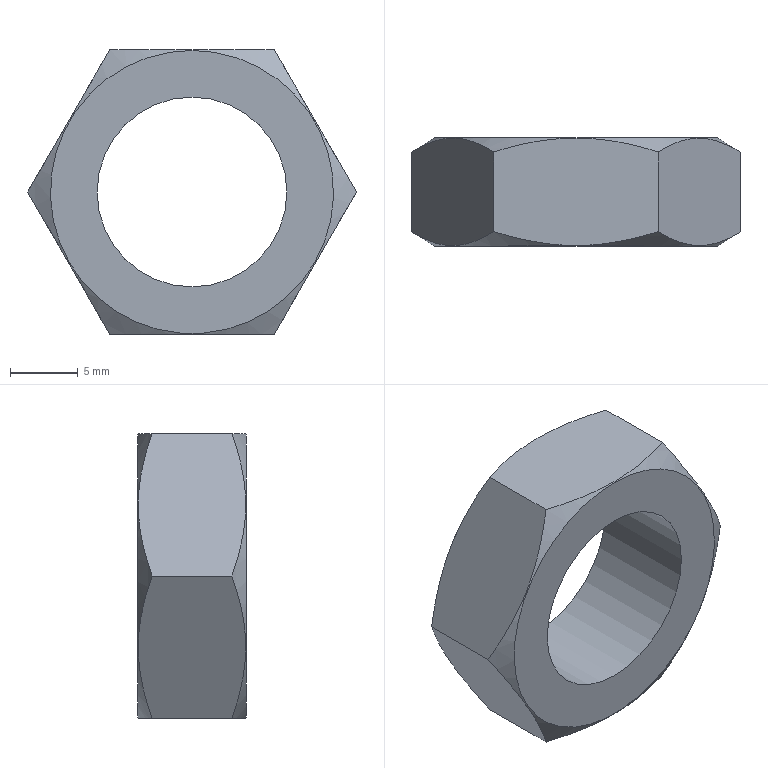Part | STEP file | 1-55.6 | 1 solid | 11 faces | box 24.249 x 8 x 21 mm | volume 1799 mm3 | plane 8 | cone 2 | cylinder 1 | commonest cylinder face diameters 14 x1
STEP:
#1=CARTESIAN_POINT('',(0.,0.,0.));
#2=DIRECTION('',(0.,0.,1.));
#3=DIRECTION('',(1.,0.,0.));
#4=AXIS2_PLACEMENT_3D('',#1,#2,#3);
#5=CARTESIAN_POINT('',(7.,4.,0.));
#6=VERTEX_POINT('',#5);
#7=CARTESIAN_POINT('',(7.,-4.,0.));
#8=VERTEX_POINT('',#7);
#9=CARTESIAN_POINT('',(7.,4.,0.));
#10=DIRECTION('',(0.,-1.,0.));
#11=VECTOR('',#10,1.);
#12=LINE('',#9,#11);
#13=CARTESIAN_POINT('',(0.,4.,0.));
#14=DIRECTION('',(0.,-1.,0.));
#15=DIRECTION('',(1.,0.,0.));
#16=AXIS2_PLACEMENT_3D('',#13,#14,#15);
#17=CYLINDRICAL_SURFACE('',#16,7.);
#18=CARTESIAN_POINT('',(6.283,0.));
#19=DIRECTION('',(0.,1.));
#20=VECTOR('',#19,1.);
#21=LINE('',#18,#20);
#22=(GEOMETRIC_REPRESENTATION_CONTEXT(2)PARAMETRIC_REPRESENTATION_CONTEXT()REPRESENTATION_CONTEXT('',''));
#23=DEFINITIONAL_REPRESENTATION('',(#21),#22);
#24=PCURVE('',#17,#23);
#25=CARTESIAN_POINT('',(0.,0.));
#26=DIRECTION('',(0.,1.));
#27=VECTOR('',#26,1.);
#28=LINE('',#25,#27);
#29=(GEOMETRIC_REPRESENTATION_CONTEXT(2)PARAMETRIC_REPRESENTATION_CONTEXT()REPRESENTATION_CONTEXT('',''));
#30=DEFINITIONAL_REPRESENTATION('',(#28),#29);
#31=PCURVE('',#17,#30);
#32=SEAM_CURVE('',#12,(#24,#31),.PCURVE_S1.);
#33=EDGE_CURVE('',#6,#8,#32,.T.);
#34=ORIENTED_EDGE('',*,*,#33,.T.);
#35=CARTESIAN_POINT('',(0.,-4.,0.));
#36=DIRECTION('',(0.,1.,0.));
#37=DIRECTION('',(1.,0.,0.));
#38=AXIS2_PLACEMENT_3D('',#35,#36,#37);
#39=CIRCLE('',#38,7.);
#40=CARTESIAN_POINT('',(6.283,8.));
#41=DIRECTION('',(-1.,0.));
#42=VECTOR('',#41,1.);
#43=LINE('',#40,#42);
#44=(GEOMETRIC_REPRESENTATION_CONTEXT(2)PARAMETRIC_REPRESENTATION_CONTEXT()REPRESENTATION_CONTEXT('',''));
#45=DEFINITIONAL_REPRESENTATION('',(#43),#44);
#46=PCURVE('',#17,#45);
#47=CARTESIAN_POINT('',(0.,-4.,1.624));
#48=DIRECTION('',(0.,-1.,0.));
#49=DIRECTION('',(1.,0.,0.));
#50=AXIS2_PLACEMENT_3D('',#47,#48,#49);
#51=PLANE('',#50);
#52=CARTESIAN_POINT('',(7.,-1.624));
#53=CARTESIAN_POINT('',(7.,-13.749));
#54=CARTESIAN_POINT('',(-3.5,-7.687));
#55=CARTESIAN_POINT('',(-14.,-1.624));
#56=CARTESIAN_POINT('',(-3.5,4.438));
#57=CARTESIAN_POINT('',(7.,10.5));
#58=CARTESIAN_POINT('',(7.,-1.624));
#59=(BOUNDED_CURVE()B_SPLINE_CURVE(2,(#52,#53,#54,#55,#56,#57,#58),.UNSPECIFIED.,.T.,.F.)B_SPLINE_CURVE_WITH_KNOTS((1,2,2,2,2,1),(-2.094,0.,2.094,4.189,6.283,8.378),.UNSPECIFIED.)CURVE()GEOMETRIC_REPRESENTATION_ITEM()RATIONAL_B_SPLINE_CURVE((1.,0.5,1.,0.5,1.,0.5,1.))REPRESENTATION_ITEM(''));
#60=(GEOMETRIC_REPRESENTATION_CONTEXT(2)PARAMETRIC_REPRESENTATION_CONTEXT()REPRESENTATION_CONTEXT('',''));
#61=DEFINITIONAL_REPRESENTATION('',(#59),#60);
#62=PCURVE('',#51,#61);
#63=SURFACE_CURVE('',#39,(#46,#62),.PCURVE_S1.);
#64=EDGE_CURVE('',#8,#8,#63,.T.);
#65=ORIENTED_EDGE('',*,*,#64,.T.);
#66=ORIENTED_EDGE('',*,*,#33,.F.);
#67=CARTESIAN_POINT('',(0.,4.,0.));
#68=DIRECTION('',(0.,1.,0.));
#69=DIRECTION('',(1.,0.,0.));
#70=AXIS2_PLACEMENT_3D('',#67,#68,#69);
#71=CIRCLE('',#70,7.);
#72=CARTESIAN_POINT('',(6.283,0.));
#73=DIRECTION('',(-1.,0.));
#74=VECTOR('',#73,1.);
#75=LINE('',#72,#74);
#76=(GEOMETRIC_REPRESENTATION_CONTEXT(2)PARAMETRIC_REPRESENTATION_CONTEXT()REPRESENTATION_CONTEXT('',''));
#77=DEFINITIONAL_REPRESENTATION('',(#75),#76);
#78=PCURVE('',#17,#77);
#79=CARTESIAN_POINT('',(0.,4.,1.624));
#80=DIRECTION('',(0.,-1.,0.));
#81=DIRECTION('',(1.,0.,0.));
#82=AXIS2_PLACEMENT_3D('',#79,#80,#81);
#83=PLANE('',#82);
#84=CARTESIAN_POINT('',(7.,-1.624));
#85=CARTESIAN_POINT('',(7.,-13.749));
#86=CARTESIAN_POINT('',(-3.5,-7.687));
#87=CARTESIAN_POINT('',(-14.,-1.624));
#88=CARTESIAN_POINT('',(-3.5,4.438));
#89=CARTESIAN_POINT('',(7.,10.5));
#90=CARTESIAN_POINT('',(7.,-1.624));
#91=(BOUNDED_CURVE()B_SPLINE_CURVE(2,(#84,#85,#86,#87,#88,#89,#90),.UNSPECIFIED.,.T.,.F.)B_SPLINE_CURVE_WITH_KNOTS((1,2,2,2,2,1),(-2.094,0.,2.094,4.189,6.283,8.378),.UNSPECIFIED.)CURVE()GEOMETRIC_REPRESENTATION_ITEM()RATIONAL_B_SPLINE_CURVE((1.,0.5,1.,0.5,1.,0.5,1.))REPRESENTATION_ITEM(''));
#92=(GEOMETRIC_REPRESENTATION_CONTEXT(2)PARAMETRIC_REPRESENTATION_CONTEXT()REPRESENTATION_CONTEXT('',''));
#93=DEFINITIONAL_REPRESENTATION('',(#91),#92);
#94=PCURVE('',#83,#93);
#95=SURFACE_CURVE('',#71,(#78,#94),.PCURVE_S1.);
#96=EDGE_CURVE('',#6,#6,#95,.T.);
#97=ORIENTED_EDGE('',*,*,#96,.F.);
#98=EDGE_LOOP('',(#34,#65,#66,#97));
#99=FACE_BOUND('',#98,.F.);
#100=ADVANCED_FACE('',(#99),#17,.F.);
#101=CARTESIAN_POINT('',(0.,4.,10.441));
#102=VERTEX_POINT('',#101);
#103=CARTESIAN_POINT('',(0.,4.,0.));
#104=DIRECTION('',(0.,1.,0.));
#105=DIRECTION('',(0.,0.,1.));
#106=AXIS2_PLACEMENT_3D('',#103,#104,#105);
#107=CIRCLE('',#106,10.441);
#108=CARTESIAN_POINT('',(0.,8.817));
#109=CARTESIAN_POINT('',(18.085,8.817));
#110=CARTESIAN_POINT('',(9.042,-6.845));
#111=CARTESIAN_POINT('',(0.,-22.507));
#112=CARTESIAN_POINT('',(-9.042,-6.845));
#113=CARTESIAN_POINT('',(-18.085,8.817));
#114=CARTESIAN_POINT('',(0.,8.817));
#115=(BOUNDED_CURVE()B_SPLINE_CURVE(2,(#108,#109,#110,#111,#112,#113,#114),.UNSPECIFIED.,.T.,.F.)B_SPLINE_CURVE_WITH_KNOTS((1,2,2,2,2,1),(-2.094,0.,2.094,4.189,6.283,8.378),.UNSPECIFIED.)CURVE()GEOMETRIC_REPRESENTATION_ITEM()RATIONAL_B_SPLINE_CURVE((1.,0.5,1.,0.5,1.,0.5,1.))REPRESENTATION_ITEM(''));
#116=(GEOMETRIC_REPRESENTATION_CONTEXT(2)PARAMETRIC_REPRESENTATION_CONTEXT()REPRESENTATION_CONTEXT('',''));
#117=DEFINITIONAL_REPRESENTATION('',(#115),#116);
#118=PCURVE('',#83,#117);
#119=CARTESIAN_POINT('',(0.,4.,0.));
#120=DIRECTION('',(0.,-1.,0.));
#121=DIRECTION('',(0.,0.,1.));
#122=AXIS2_PLACEMENT_3D('',#119,#120,#121);
#123=CONICAL_SURFACE('',#122,10.441,1.008);
#124=CARTESIAN_POINT('',(6.283,0.));
#125=DIRECTION('',(-1.,0.));
#126=VECTOR('',#125,1.);
#127=LINE('',#124,#126);
#128=(GEOMETRIC_REPRESENTATION_CONTEXT(2)PARAMETRIC_REPRESENTATION_CONTEXT()REPRESENTATION_CONTEXT('',''));
#129=DEFINITIONAL_REPRESENTATION('',(#127),#128);
#130=PCURVE('',#123,#129);
#131=SURFACE_CURVE('',#107,(#118,#130),.PCURVE_S1.);
#132=EDGE_CURVE('',#102,#102,#131,.T.);
#133=ORIENTED_EDGE('',*,*,#132,.F.);
#134=EDGE_LOOP('',(#133));
#135=FACE_BOUND('',#134,.F.);
#136=ORIENTED_EDGE('',*,*,#96,.T.);
#137=EDGE_LOOP('',(#136));
#138=FACE_BOUND('',#137,.F.);
#139=ADVANCED_FACE('',(#135,#138),#83,.F.);
#140=CARTESIAN_POINT('',(0.,-4.,10.441));
#141=VERTEX_POINT('',#140);
#142=CARTESIAN_POINT('',(0.,-4.,0.));
#143=DIRECTION('',(0.,1.,0.));
#144=DIRECTION('',(0.,0.,1.));
#145=AXIS2_PLACEMENT_3D('',#142,#143,#144);
#146=CIRCLE('',#145,10.441);
#147=CARTESIAN_POINT('',(0.,8.817));
#148=CARTESIAN_POINT('',(18.085,8.817));
#149=CARTESIAN_POINT('',(9.042,-6.845));
#150=CARTESIAN_POINT('',(0.,-22.507));
#151=CARTESIAN_POINT('',(-9.042,-6.845));
#152=CARTESIAN_POINT('',(-18.085,8.817));
#153=CARTESIAN_POINT('',(0.,8.817));
#154=(BOUNDED_CURVE()B_SPLINE_CURVE(2,(#147,#148,#149,#150,#151,#152,#153),.UNSPECIFIED.,.T.,.F.)B_SPLINE_CURVE_WITH_KNOTS((1,2,2,2,2,1),(-2.094,0.,2.094,4.189,6.283,8.378),.UNSPECIFIED.)CURVE()GEOMETRIC_REPRESENTATION_ITEM()RATIONAL_B_SPLINE_CURVE((1.,0.5,1.,0.5,1.,0.5,1.))REPRESENTATION_ITEM(''));
#155=(GEOMETRIC_REPRESENTATION_CONTEXT(2)PARAMETRIC_REPRESENTATION_CONTEXT()REPRESENTATION_CONTEXT('',''));
#156=DEFINITIONAL_REPRESENTATION('',(#154),#155);
#157=PCURVE('',#51,#156);
#158=CARTESIAN_POINT('',(0.,-4.,0.));
#159=DIRECTION('',(0.,1.,0.));
#160=DIRECTION('',(0.,0.,1.));
#161=AXIS2_PLACEMENT_3D('',#158,#159,#160);
#162=CONICAL_SURFACE('',#161,10.441,1.008);
#163=CARTESIAN_POINT('',(0.,0.));
#164=DIRECTION('',(1.,0.));
#165=VECTOR('',#164,1.);
#166=LINE('',#163,#165);
#167=(GEOMETRIC_REPRESENTATION_CONTEXT(2)PARAMETRIC_REPRESENTATION_CONTEXT()REPRESENTATION_CONTEXT('',''));
#168=DEFINITIONAL_REPRESENTATION('',(#166),#167);
#169=PCURVE('',#162,#168);
#170=SURFACE_CURVE('',#146,(#157,#169),.PCURVE_S1.);
#171=EDGE_CURVE('',#141,#141,#170,.T.);
#172=ORIENTED_EDGE('',*,*,#171,.F.);
#173=EDGE_LOOP('',(#172));
#174=FACE_BOUND('',#173,.T.);
#175=ORIENTED_EDGE('',*,*,#64,.T.);
#176=EDGE_LOOP('',(#175));
#177=FACE_BOUND('',#176,.T.);
#178=ADVANCED_FACE('',(#174,#177),#51,.T.);
#179=CARTESIAN_POINT('',(12.124,2.938,0.));
#180=VERTEX_POINT('',#179);
#181=CARTESIAN_POINT('',(12.124,-2.938,0.));
#182=VERTEX_POINT('',#181);
#183=CARTESIAN_POINT('',(12.124,2.938,0.));
#184=DIRECTION('',(0.,-1.,0.));
#185=VECTOR('',#184,1.);
#186=LINE('',#183,#185);
#187=CARTESIAN_POINT('',(9.093,0.,5.25));
#188=DIRECTION('',(0.866,0.,0.5));
#189=DIRECTION('',(-0.5,0.,0.866));
#190=AXIS2_PLACEMENT_3D('',#187,#188,#189);
#191=PLANE('',#190);
#192=CARTESIAN_POINT('',(-6.062,-2.938));
#193=DIRECTION('',(0.,1.));
#194=VECTOR('',#193,1.);
#195=LINE('',#192,#194);
#196=(GEOMETRIC_REPRESENTATION_CONTEXT(2)PARAMETRIC_REPRESENTATION_CONTEXT()REPRESENTATION_CONTEXT('',''));
#197=DEFINITIONAL_REPRESENTATION('',(#195),#196);
#198=PCURVE('',#191,#197);
#199=CARTESIAN_POINT('',(9.093,0.,-5.25));
#200=DIRECTION('',(0.866,0.,-0.5));
#201=DIRECTION('',(0.5,0.,0.866));
#202=AXIS2_PLACEMENT_3D('',#199,#200,#201);
#203=PLANE('',#202);
#204=CARTESIAN_POINT('',(6.062,-2.938));
#205=DIRECTION('',(0.,1.));
#206=VECTOR('',#205,1.);
#207=LINE('',#204,#206);
#208=(GEOMETRIC_REPRESENTATION_CONTEXT(2)PARAMETRIC_REPRESENTATION_CONTEXT()REPRESENTATION_CONTEXT('',''));
#209=DEFINITIONAL_REPRESENTATION('',(#207),#208);
#210=PCURVE('',#203,#209);
#211=SURFACE_CURVE('',#186,(#198,#210),.PCURVE_S1.);
#212=EDGE_CURVE('',#180,#182,#211,.T.);
#213=ORIENTED_EDGE('',*,*,#212,.F.);
#214=CARTESIAN_POINT('',(6.062,2.938,10.5));
#215=VERTEX_POINT('',#214);
#216=CARTESIAN_POINT('',(6.062,2.938,10.5));
#217=CARTESIAN_POINT('',(9.093,4.85,5.25));
#218=CARTESIAN_POINT('',(12.124,2.938,0.));
#219=(BOUNDED_CURVE()B_SPLINE_CURVE(2,(#216,#217,#218),.UNSPECIFIED.,.F.,.F.)B_SPLINE_CURVE_WITH_KNOTS((3,3),(0.,1.),.PIECEWISE_BEZIER_KNOTS.)CURVE()GEOMETRIC_REPRESENTATION_ITEM()RATIONAL_B_SPLINE_CURVE((1.206,1.392,1.206))REPRESENTATION_ITEM(''));
#220=CARTESIAN_POINT('',(6.062,-2.938));
#221=CARTESIAN_POINT('',(0.,-4.85));
#222=CARTESIAN_POINT('',(-6.062,-2.938));
#223=(BOUNDED_CURVE()B_SPLINE_CURVE(2,(#220,#221,#222),.UNSPECIFIED.,.F.,.F.)B_SPLINE_CURVE_WITH_KNOTS((3,3),(0.,1.),.PIECEWISE_BEZIER_KNOTS.)CURVE()GEOMETRIC_REPRESENTATION_ITEM()RATIONAL_B_SPLINE_CURVE((1.206,1.392,1.206))REPRESENTATION_ITEM(''));
#224=(GEOMETRIC_REPRESENTATION_CONTEXT(2)PARAMETRIC_REPRESENTATION_CONTEXT()REPRESENTATION_CONTEXT('',''));
#225=DEFINITIONAL_REPRESENTATION('',(#223),#224);
#226=PCURVE('',#191,#225);
#227=CARTESIAN_POINT('',(5.76,1.062));
#228=CARTESIAN_POINT('',(5.744,0.9946));
#229=CARTESIAN_POINT('',(5.714,0.8688));
#230=CARTESIAN_POINT('',(5.668,0.7023));
#231=CARTESIAN_POINT('',(5.621,0.5566));
#232=CARTESIAN_POINT('',(5.574,0.4305));
#233=CARTESIAN_POINT('',(5.526,0.3231));
#234=CARTESIAN_POINT('',(5.478,0.2336));
#235=CARTESIAN_POINT('',(5.43,0.1612));
#236=CARTESIAN_POINT('',(5.382,0.1054));
#237=CARTESIAN_POINT('',(5.333,0.06584));
#238=CARTESIAN_POINT('',(5.285,0.04222));
#239=CARTESIAN_POINT('',(5.236,0.03437));
#240=CARTESIAN_POINT('',(5.187,0.04222));
#241=CARTESIAN_POINT('',(5.139,0.06584));
#242=CARTESIAN_POINT('',(5.09,0.1054));
#243=CARTESIAN_POINT('',(5.042,0.1612));
#244=CARTESIAN_POINT('',(4.994,0.2336));
#245=CARTESIAN_POINT('',(4.946,0.3231));
#246=CARTESIAN_POINT('',(4.898,0.4305));
#247=CARTESIAN_POINT('',(4.851,0.5566));
#248=CARTESIAN_POINT('',(4.804,0.7023));
#249=CARTESIAN_POINT('',(4.758,0.8688));
#250=CARTESIAN_POINT('',(4.728,0.9946));
#251=CARTESIAN_POINT('',(4.712,1.062));
#252=B_SPLINE_CURVE_WITH_KNOTS('',3,(#227,#228,#229,#230,#231,#232,#233,#234,#235,#236,#237,#238,#239,#240,#241,#242,#243,#244,#245,#246,#247,#248,#249,#250,#251),.UNSPECIFIED.,.F.,.F.,(4,1,1,1,1,1,1,1,1,1,1,1,1,1,1,1,1,1,1,1,1,1,4),(0.,0.04545,0.09091,0.1364,0.1818,0.2273,0.2727,0.3182,0.3636,0.4091,0.4545,0.5,0.5455,0.5909,0.6364,0.6818,0.7273,0.7727,0.8182,0.8636,0.9091,0.9545,1.),.QUASI_UNIFORM_KNOTS.);
#253=(GEOMETRIC_REPRESENTATION_CONTEXT(2)PARAMETRIC_REPRESENTATION_CONTEXT()REPRESENTATION_CONTEXT('',''));
#254=DEFINITIONAL_REPRESENTATION('',(#252),#253);
#255=PCURVE('',#123,#254);
#256=SURFACE_CURVE('',#219,(#226,#255),.PCURVE_S1.);
#257=EDGE_CURVE('',#215,#180,#256,.T.);
#258=ORIENTED_EDGE('',*,*,#257,.F.);
#259=CARTESIAN_POINT('',(6.062,-2.938,10.5));
#260=VERTEX_POINT('',#259);
#261=CARTESIAN_POINT('',(6.062,2.938,10.5));
#262=DIRECTION('',(0.,-1.,0.));
#263=VECTOR('',#262,1.);
#264=LINE('',#261,#263);
#265=CARTESIAN_POINT('',(6.062,-2.938));
#266=DIRECTION('',(0.,1.));
#267=VECTOR('',#266,1.);
#268=LINE('',#265,#267);
#269=(GEOMETRIC_REPRESENTATION_CONTEXT(2)PARAMETRIC_REPRESENTATION_CONTEXT()REPRESENTATION_CONTEXT('',''));
#270=DEFINITIONAL_REPRESENTATION('',(#268),#269);
#271=PCURVE('',#191,#270);
#272=CARTESIAN_POINT('',(0.,0.,10.5));
#273=DIRECTION('',(0.,0.,1.));
#274=DIRECTION('',(-1.,0.,0.));
#275=AXIS2_PLACEMENT_3D('',#272,#273,#274);
#276=PLANE('',#275);
#277=CARTESIAN_POINT('',(-6.062,-2.938));
#278=DIRECTION('',(0.,1.));
#279=VECTOR('',#278,1.);
#280=LINE('',#277,#279);
#281=(GEOMETRIC_REPRESENTATION_CONTEXT(2)PARAMETRIC_REPRESENTATION_CONTEXT()REPRESENTATION_CONTEXT('',''));
#282=DEFINITIONAL_REPRESENTATION('',(#280),#281);
#283=PCURVE('',#276,#282);
#284=SURFACE_CURVE('',#264,(#271,#283),.PCURVE_S1.);
#285=EDGE_CURVE('',#215,#260,#284,.T.);
#286=ORIENTED_EDGE('',*,*,#285,.T.);
#287=CARTESIAN_POINT('',(12.124,-2.938,0.));
#288=CARTESIAN_POINT('',(9.093,-4.85,5.25));
#289=CARTESIAN_POINT('',(6.062,-2.938,10.5));
#290=(BOUNDED_CURVE()B_SPLINE_CURVE(2,(#287,#288,#289),.UNSPECIFIED.,.F.,.F.)B_SPLINE_CURVE_WITH_KNOTS((3,3),(0.,1.),.PIECEWISE_BEZIER_KNOTS.)CURVE()GEOMETRIC_REPRESENTATION_ITEM()RATIONAL_B_SPLINE_CURVE((1.206,1.392,1.206))REPRESENTATION_ITEM(''));
#291=CARTESIAN_POINT('',(-6.062,2.938));
#292=CARTESIAN_POINT('',(0.,4.85));
#293=CARTESIAN_POINT('',(6.062,2.938));
#294=(BOUNDED_CURVE()B_SPLINE_CURVE(2,(#291,#292,#293),.UNSPECIFIED.,.F.,.F.)B_SPLINE_CURVE_WITH_KNOTS((3,3),(0.,1.),.PIECEWISE_BEZIER_KNOTS.)CURVE()GEOMETRIC_REPRESENTATION_ITEM()RATIONAL_B_SPLINE_CURVE((1.206,1.392,1.206))REPRESENTATION_ITEM(''));
#295=(GEOMETRIC_REPRESENTATION_CONTEXT(2)PARAMETRIC_REPRESENTATION_CONTEXT()REPRESENTATION_CONTEXT('',''));
#296=DEFINITIONAL_REPRESENTATION('',(#294),#295);
#297=PCURVE('',#191,#296);
#298=CARTESIAN_POINT('',(1.571,1.062));
#299=CARTESIAN_POINT('',(1.556,0.9946));
#300=CARTESIAN_POINT('',(1.525,0.8688));
#301=CARTESIAN_POINT('',(1.479,0.7023));
#302=CARTESIAN_POINT('',(1.432,0.5566));
#303=CARTESIAN_POINT('',(1.385,0.4305));
#304=CARTESIAN_POINT('',(1.338,0.3231));
#305=CARTESIAN_POINT('',(1.29,0.2336));
#306=CARTESIAN_POINT('',(1.241,0.1612));
#307=CARTESIAN_POINT('',(1.193,0.1054));
#308=CARTESIAN_POINT('',(1.145,0.06584));
#309=CARTESIAN_POINT('',(1.096,0.04222));
#310=CARTESIAN_POINT('',(1.047,0.03437));
#311=CARTESIAN_POINT('',(0.9985,0.04222));
#312=CARTESIAN_POINT('',(0.9498,0.06584));
#313=CARTESIAN_POINT('',(0.9013,0.1054));
#314=CARTESIAN_POINT('',(0.8529,0.1612));
#315=CARTESIAN_POINT('',(0.8048,0.2336));
#316=CARTESIAN_POINT('',(0.7569,0.3231));
#317=CARTESIAN_POINT('',(0.7094,0.4305));
#318=CARTESIAN_POINT('',(0.6622,0.5566));
#319=CARTESIAN_POINT('',(0.6155,0.7023));
#320=CARTESIAN_POINT('',(0.5692,0.8688));
#321=CARTESIAN_POINT('',(0.5388,0.9946));
#322=CARTESIAN_POINT('',(0.5236,1.062));
#323=B_SPLINE_CURVE_WITH_KNOTS('',3,(#298,#299,#300,#301,#302,#303,#304,#305,#306,#307,#308,#309,#310,#311,#312,#313,#314,#315,#316,#317,#318,#319,#320,#321,#322),.UNSPECIFIED.,.F.,.F.,(4,1,1,1,1,1,1,1,1,1,1,1,1,1,1,1,1,1,1,1,1,1,4),(0.,0.04545,0.09091,0.1364,0.1818,0.2273,0.2727,0.3182,0.3636,0.4091,0.4545,0.5,0.5455,0.5909,0.6364,0.6818,0.7273,0.7727,0.8182,0.8636,0.9091,0.9545,1.),.QUASI_UNIFORM_KNOTS.);
#324=(GEOMETRIC_REPRESENTATION_CONTEXT(2)PARAMETRIC_REPRESENTATION_CONTEXT()REPRESENTATION_CONTEXT('',''));
#325=DEFINITIONAL_REPRESENTATION('',(#323),#324);
#326=PCURVE('',#162,#325);
#327=SURFACE_CURVE('',#290,(#297,#326),.PCURVE_S1.);
#328=EDGE_CURVE('',#182,#260,#327,.T.);
#329=ORIENTED_EDGE('',*,*,#328,.F.);
#330=EDGE_LOOP('',(#213,#258,#286,#329));
#331=FACE_BOUND('',#330,.T.);
#332=ADVANCED_FACE('',(#331),#191,.T.);
#333=ORIENTED_EDGE('',*,*,#285,.F.);
#334=CARTESIAN_POINT('',(0.,3.963,10.5));
#335=VERTEX_POINT('',#334);
#336=CARTESIAN_POINT('',(0.,3.963,10.5));
#337=CARTESIAN_POINT('',(2.813,3.963,10.5));
#338=CARTESIAN_POINT('',(6.062,2.938,10.5));
#339=(BOUNDED_CURVE()B_SPLINE_CURVE(2,(#336,#337,#338),.UNSPECIFIED.,.F.,.F.)B_SPLINE_CURVE_WITH_KNOTS((3,3),(0.,1.),.PIECEWISE_BEZIER_KNOTS.)CURVE()GEOMETRIC_REPRESENTATION_ITEM()RATIONAL_B_SPLINE_CURVE((1.299,1.299,1.206))REPRESENTATION_ITEM(''));
#340=CARTESIAN_POINT('',(0.,-3.963));
#341=CARTESIAN_POINT('',(-2.813,-3.963));
#342=CARTESIAN_POINT('',(-6.062,-2.938));
#343=(BOUNDED_CURVE()B_SPLINE_CURVE(2,(#340,#341,#342),.UNSPECIFIED.,.F.,.F.)B_SPLINE_CURVE_WITH_KNOTS((3,3),(0.,1.),.PIECEWISE_BEZIER_KNOTS.)CURVE()GEOMETRIC_REPRESENTATION_ITEM()RATIONAL_B_SPLINE_CURVE((1.299,1.299,1.206))REPRESENTATION_ITEM(''));
#344=(GEOMETRIC_REPRESENTATION_CONTEXT(2)PARAMETRIC_REPRESENTATION_CONTEXT()REPRESENTATION_CONTEXT('',''));
#345=DEFINITIONAL_REPRESENTATION('',(#343),#344);
#346=PCURVE('',#276,#345);
#347=CARTESIAN_POINT('',(6.283,0.03698));
#348=CARTESIAN_POINT('',(6.275,0.03698));
#349=CARTESIAN_POINT('',(6.259,0.03829));
#350=CARTESIAN_POINT('',(6.234,0.04419));
#351=CARTESIAN_POINT('',(6.21,0.05403));
#352=CARTESIAN_POINT('',(6.186,0.06783));
#353=CARTESIAN_POINT('',(6.162,0.08562));
#354=CARTESIAN_POINT('',(6.137,0.1074));
#355=CARTESIAN_POINT('',(6.113,0.1333));
#356=CARTESIAN_POINT('',(6.089,0.1632));
#357=CARTESIAN_POINT('',(6.065,0.1974));
#358=CARTESIAN_POINT('',(6.041,0.2357));
#359=CARTESIAN_POINT('',(6.017,0.2783));
#360=CARTESIAN_POINT('',(5.993,0.3253));
#361=CARTESIAN_POINT('',(5.969,0.3768));
#362=CARTESIAN_POINT('',(5.945,0.4328));
#363=CARTESIAN_POINT('',(5.922,0.4935));
#364=CARTESIAN_POINT('',(5.898,0.559));
#365=CARTESIAN_POINT('',(5.875,0.6294));
#366=CARTESIAN_POINT('',(5.852,0.7049));
#367=CARTESIAN_POINT('',(5.828,0.7855));
#368=CARTESIAN_POINT('',(5.805,0.8716));
#369=CARTESIAN_POINT('',(5.782,0.9632));
#370=CARTESIAN_POINT('',(5.767,1.028));
#371=CARTESIAN_POINT('',(5.76,1.062));
#372=B_SPLINE_CURVE_WITH_KNOTS('',3,(#347,#348,#349,#350,#351,#352,#353,#354,#355,#356,#357,#358,#359,#360,#361,#362,#363,#364,#365,#366,#367,#368,#369,#370,#371),.UNSPECIFIED.,.F.,.F.,(4,1,1,1,1,1,1,1,1,1,1,1,1,1,1,1,1,1,1,1,1,1,4),(0.,0.04545,0.09091,0.1364,0.1818,0.2273,0.2727,0.3182,0.3636,0.4091,0.4545,0.5,0.5455,0.5909,0.6364,0.6818,0.7273,0.7727,0.8182,0.8636,0.9091,0.9545,1.),.QUASI_UNIFORM_KNOTS.);
#373=(GEOMETRIC_REPRESENTATION_CONTEXT(2)PARAMETRIC_REPRESENTATION_CONTEXT()REPRESENTATION_CONTEXT('',''));
#374=DEFINITIONAL_REPRESENTATION('',(#372),#373);
#375=PCURVE('',#123,#374);
#376=SURFACE_CURVE('',#339,(#346,#375),.PCURVE_S1.);
#377=EDGE_CURVE('',#335,#215,#376,.T.);
#378=ORIENTED_EDGE('',*,*,#377,.F.);
#379=CARTESIAN_POINT('',(-6.062,2.938,10.5));
#380=VERTEX_POINT('',#379);
#381=CARTESIAN_POINT('',(-6.062,2.938,10.5));
#382=CARTESIAN_POINT('',(-2.813,3.963,10.5));
#383=CARTESIAN_POINT('',(0.,3.963,10.5));
#384=(BOUNDED_CURVE()B_SPLINE_CURVE(2,(#381,#382,#383),.UNSPECIFIED.,.F.,.F.)B_SPLINE_CURVE_WITH_KNOTS((3,3),(0.,1.),.PIECEWISE_BEZIER_KNOTS.)CURVE()GEOMETRIC_REPRESENTATION_ITEM()RATIONAL_B_SPLINE_CURVE((1.206,1.299,1.299))REPRESENTATION_ITEM(''));
#385=CARTESIAN_POINT('',(6.062,-2.938));
#386=CARTESIAN_POINT('',(2.813,-3.963));
#387=CARTESIAN_POINT('',(0.,-3.963));
#388=(BOUNDED_CURVE()B_SPLINE_CURVE(2,(#385,#386,#387),.UNSPECIFIED.,.F.,.F.)B_SPLINE_CURVE_WITH_KNOTS((3,3),(0.,1.),.PIECEWISE_BEZIER_KNOTS.)CURVE()GEOMETRIC_REPRESENTATION_ITEM()RATIONAL_B_SPLINE_CURVE((1.206,1.299,1.299))REPRESENTATION_ITEM(''));
#389=(GEOMETRIC_REPRESENTATION_CONTEXT(2)PARAMETRIC_REPRESENTATION_CONTEXT()REPRESENTATION_CONTEXT('',''));
#390=DEFINITIONAL_REPRESENTATION('',(#388),#389);
#391=PCURVE('',#276,#390);
#392=CARTESIAN_POINT('',(0.5236,1.062));
#393=CARTESIAN_POINT('',(0.516,1.028));
#394=CARTESIAN_POINT('',(0.5008,0.9632));
#395=CARTESIAN_POINT('',(0.4779,0.8716));
#396=CARTESIAN_POINT('',(0.4548,0.7855));
#397=CARTESIAN_POINT('',(0.4317,0.7049));
#398=CARTESIAN_POINT('',(0.4084,0.6294));
#399=CARTESIAN_POINT('',(0.3849,0.559));
#400=CARTESIAN_POINT('',(0.3614,0.4935));
#401=CARTESIAN_POINT('',(0.3378,0.4328));
#402=CARTESIAN_POINT('',(0.3141,0.3768));
#403=CARTESIAN_POINT('',(0.2903,0.3253));
#404=CARTESIAN_POINT('',(0.2664,0.2783));
#405=CARTESIAN_POINT('',(0.2424,0.2357));
#406=CARTESIAN_POINT('',(0.2184,0.1974));
#407=CARTESIAN_POINT('',(0.1943,0.1632));
#408=CARTESIAN_POINT('',(0.1701,0.1333));
#409=CARTESIAN_POINT('',(0.1459,0.1074));
#410=CARTESIAN_POINT('',(0.1217,0.08562));
#411=CARTESIAN_POINT('',(0.09736,0.06783));
#412=CARTESIAN_POINT('',(0.07305,0.05403));
#413=CARTESIAN_POINT('',(0.04871,0.04419));
#414=CARTESIAN_POINT('',(0.02436,0.03829));
#415=CARTESIAN_POINT('',(0.00812,0.03698));
#416=CARTESIAN_POINT('',(0.,0.03698));
#417=B_SPLINE_CURVE_WITH_KNOTS('',3,(#392,#393,#394,#395,#396,#397,#398,#399,#400,#401,#402,#403,#404,#405,#406,#407,#408,#409,#410,#411,#412,#413,#414,#415,#416),.UNSPECIFIED.,.F.,.F.,(4,1,1,1,1,1,1,1,1,1,1,1,1,1,1,1,1,1,1,1,1,1,4),(0.,0.04545,0.09091,0.1364,0.1818,0.2273,0.2727,0.3182,0.3636,0.4091,0.4545,0.5,0.5455,0.5909,0.6364,0.6818,0.7273,0.7727,0.8182,0.8636,0.9091,0.9545,1.),.QUASI_UNIFORM_KNOTS.);
#418=(GEOMETRIC_REPRESENTATION_CONTEXT(2)PARAMETRIC_REPRESENTATION_CONTEXT()REPRESENTATION_CONTEXT('',''));
#419=DEFINITIONAL_REPRESENTATION('',(#417),#418);
#420=PCURVE('',#123,#419);
#421=SURFACE_CURVE('',#384,(#391,#420),.PCURVE_S1.);
#422=EDGE_CURVE('',#380,#335,#421,.T.);
#423=ORIENTED_EDGE('',*,*,#422,.F.);
#424=CARTESIAN_POINT('',(-6.062,-2.938,10.5));
#425=VERTEX_POINT('',#424);
#426=CARTESIAN_POINT('',(-6.062,2.938,10.5));
#427=DIRECTION('',(0.,-1.,0.));
#428=VECTOR('',#427,1.);
#429=LINE('',#426,#428);
#430=CARTESIAN_POINT('',(6.062,-2.938));
#431=DIRECTION('',(0.,1.));
#432=VECTOR('',#431,1.);
#433=LINE('',#430,#432);
#434=(GEOMETRIC_REPRESENTATION_CONTEXT(2)PARAMETRIC_REPRESENTATION_CONTEXT()REPRESENTATION_CONTEXT('',''));
#435=DEFINITIONAL_REPRESENTATION('',(#433),#434);
#436=PCURVE('',#276,#435);
#437=CARTESIAN_POINT('',(-9.093,0.,5.25));
#438=DIRECTION('',(-0.866,0.,0.5));
#439=DIRECTION('',(-0.5,0.,-0.866));
#440=AXIS2_PLACEMENT_3D('',#437,#438,#439);
#441=PLANE('',#440);
#442=CARTESIAN_POINT('',(-6.062,-2.938));
#443=DIRECTION('',(0.,1.));
#444=VECTOR('',#443,1.);
#445=LINE('',#442,#444);
#446=(GEOMETRIC_REPRESENTATION_CONTEXT(2)PARAMETRIC_REPRESENTATION_CONTEXT()REPRESENTATION_CONTEXT('',''));
#447=DEFINITIONAL_REPRESENTATION('',(#445),#446);
#448=PCURVE('',#441,#447);
#449=SURFACE_CURVE('',#429,(#436,#448),.PCURVE_S1.);
#450=EDGE_CURVE('',#380,#425,#449,.T.);
#451=ORIENTED_EDGE('',*,*,#450,.T.);
#452=CARTESIAN_POINT('',(0.,-3.963,10.5));
#453=VERTEX_POINT('',#452);
#454=CARTESIAN_POINT('',(0.,-3.963,10.5));
#455=CARTESIAN_POINT('',(-2.813,-3.963,10.5));
#456=CARTESIAN_POINT('',(-6.062,-2.938,10.5));
#457=(BOUNDED_CURVE()B_SPLINE_CURVE(2,(#454,#455,#456),.UNSPECIFIED.,.F.,.F.)B_SPLINE_CURVE_WITH_KNOTS((3,3),(0.,1.),.PIECEWISE_BEZIER_KNOTS.)CURVE()GEOMETRIC_REPRESENTATION_ITEM()RATIONAL_B_SPLINE_CURVE((1.299,1.299,1.206))REPRESENTATION_ITEM(''));
#458=CARTESIAN_POINT('',(0.,3.963));
#459=CARTESIAN_POINT('',(2.813,3.963));
#460=CARTESIAN_POINT('',(6.062,2.938));
#461=(BOUNDED_CURVE()B_SPLINE_CURVE(2,(#458,#459,#460),.UNSPECIFIED.,.F.,.F.)B_SPLINE_CURVE_WITH_KNOTS((3,3),(0.,1.),.PIECEWISE_BEZIER_KNOTS.)CURVE()GEOMETRIC_REPRESENTATION_ITEM()RATIONAL_B_SPLINE_CURVE((1.299,1.299,1.206))REPRESENTATION_ITEM(''));
#462=(GEOMETRIC_REPRESENTATION_CONTEXT(2)PARAMETRIC_REPRESENTATION_CONTEXT()REPRESENTATION_CONTEXT('',''));
#463=DEFINITIONAL_REPRESENTATION('',(#461),#462);
#464=PCURVE('',#276,#463);
#465=CARTESIAN_POINT('',(6.283,0.03698));
#466=CARTESIAN_POINT('',(6.275,0.03698));
#467=CARTESIAN_POINT('',(6.259,0.03829));
#468=CARTESIAN_POINT('',(6.234,0.04419));
#469=CARTESIAN_POINT('',(6.21,0.05403));
#470=CARTESIAN_POINT('',(6.186,0.06783));
#471=CARTESIAN_POINT('',(6.162,0.08562));
#472=CARTESIAN_POINT('',(6.137,0.1074));
#473=CARTESIAN_POINT('',(6.113,0.1333));
#474=CARTESIAN_POINT('',(6.089,0.1632));
#475=CARTESIAN_POINT('',(6.065,0.1974));
#476=CARTESIAN_POINT('',(6.041,0.2357));
#477=CARTESIAN_POINT('',(6.017,0.2783));
#478=CARTESIAN_POINT('',(5.993,0.3253));
#479=CARTESIAN_POINT('',(5.969,0.3768));
#480=CARTESIAN_POINT('',(5.945,0.4328));
#481=CARTESIAN_POINT('',(5.922,0.4935));
#482=CARTESIAN_POINT('',(5.898,0.559));
#483=CARTESIAN_POINT('',(5.875,0.6294));
#484=CARTESIAN_POINT('',(5.852,0.7049));
#485=CARTESIAN_POINT('',(5.828,0.7855));
#486=CARTESIAN_POINT('',(5.805,0.8716));
#487=CARTESIAN_POINT('',(5.782,0.9632));
#488=CARTESIAN_POINT('',(5.767,1.028));
#489=CARTESIAN_POINT('',(5.76,1.062));
#490=B_SPLINE_CURVE_WITH_KNOTS('',3,(#465,#466,#467,#468,#469,#470,#471,#472,#473,#474,#475,#476,#477,#478,#479,#480,#481,#482,#483,#484,#485,#486,#487,#488,#489),.UNSPECIFIED.,.F.,.F.,(4,1,1,1,1,1,1,1,1,1,1,1,1,1,1,1,1,1,1,1,1,1,4),(0.,0.04545,0.09091,0.1364,0.1818,0.2273,0.2727,0.3182,0.3636,0.4091,0.4545,0.5,0.5455,0.5909,0.6364,0.6818,0.7273,0.7727,0.8182,0.8636,0.9091,0.9545,1.),.QUASI_UNIFORM_KNOTS.);
#491=(GEOMETRIC_REPRESENTATION_CONTEXT(2)PARAMETRIC_REPRESENTATION_CONTEXT()REPRESENTATION_CONTEXT('',''));
#492=DEFINITIONAL_REPRESENTATION('',(#490),#491);
#493=PCURVE('',#162,#492);
#494=SURFACE_CURVE('',#457,(#464,#493),.PCURVE_S1.);
#495=EDGE_CURVE('',#453,#425,#494,.T.);
#496=ORIENTED_EDGE('',*,*,#495,.F.);
#497=CARTESIAN_POINT('',(6.062,-2.938,10.5));
#498=CARTESIAN_POINT('',(2.813,-3.963,10.5));
#499=CARTESIAN_POINT('',(0.,-3.963,10.5));
#500=(BOUNDED_CURVE()B_SPLINE_CURVE(2,(#497,#498,#499),.UNSPECIFIED.,.F.,.F.)B_SPLINE_CURVE_WITH_KNOTS((3,3),(0.,1.),.PIECEWISE_BEZIER_KNOTS.)CURVE()GEOMETRIC_REPRESENTATION_ITEM()RATIONAL_B_SPLINE_CURVE((1.206,1.299,1.299))REPRESENTATION_ITEM(''));
#501=CARTESIAN_POINT('',(-6.062,2.938));
#502=CARTESIAN_POINT('',(-2.813,3.963));
#503=CARTESIAN_POINT('',(0.,3.963));
#504=(BOUNDED_CURVE()B_SPLINE_CURVE(2,(#501,#502,#503),.UNSPECIFIED.,.F.,.F.)B_SPLINE_CURVE_WITH_KNOTS((3,3),(0.,1.),.PIECEWISE_BEZIER_KNOTS.)CURVE()GEOMETRIC_REPRESENTATION_ITEM()RATIONAL_B_SPLINE_CURVE((1.206,1.299,1.299))REPRESENTATION_ITEM(''));
#505=(GEOMETRIC_REPRESENTATION_CONTEXT(2)PARAMETRIC_REPRESENTATION_CONTEXT()REPRESENTATION_CONTEXT('',''));
#506=DEFINITIONAL_REPRESENTATION('',(#504),#505);
#507=PCURVE('',#276,#506);
#508=CARTESIAN_POINT('',(0.5236,1.062));
#509=CARTESIAN_POINT('',(0.516,1.028));
#510=CARTESIAN_POINT('',(0.5008,0.9632));
#511=CARTESIAN_POINT('',(0.4779,0.8716));
#512=CARTESIAN_POINT('',(0.4548,0.7855));
#513=CARTESIAN_POINT('',(0.4317,0.7049));
#514=CARTESIAN_POINT('',(0.4084,0.6294));
#515=CARTESIAN_POINT('',(0.3849,0.559));
#516=CARTESIAN_POINT('',(0.3614,0.4935));
#517=CARTESIAN_POINT('',(0.3378,0.4328));
#518=CARTESIAN_POINT('',(0.3141,0.3768));
#519=CARTESIAN_POINT('',(0.2903,0.3253));
#520=CARTESIAN_POINT('',(0.2664,0.2783));
#521=CARTESIAN_POINT('',(0.2424,0.2357));
#522=CARTESIAN_POINT('',(0.2184,0.1974));
#523=CARTESIAN_POINT('',(0.1943,0.1632));
#524=CARTESIAN_POINT('',(0.1701,0.1333));
#525=CARTESIAN_POINT('',(0.1459,0.1074));
#526=CARTESIAN_POINT('',(0.1217,0.08562));
#527=CARTESIAN_POINT('',(0.09736,0.06783));
#528=CARTESIAN_POINT('',(0.07305,0.05403));
#529=CARTESIAN_POINT('',(0.04871,0.04419));
#530=CARTESIAN_POINT('',(0.02436,0.03829));
#531=CARTESIAN_POINT('',(0.00812,0.03698));
#532=CARTESIAN_POINT('',(0.,0.03698));
#533=B_SPLINE_CURVE_WITH_KNOTS('',3,(#508,#509,#510,#511,#512,#513,#514,#515,#516,#517,#518,#519,#520,#521,#522,#523,#524,#525,#526,#527,#528,#529,#530,#531,#532),.UNSPECIFIED.,.F.,.F.,(4,1,1,1,1,1,1,1,1,1,1,1,1,1,1,1,1,1,1,1,1,1,4),(0.,0.04545,0.09091,0.1364,0.1818,0.2273,0.2727,0.3182,0.3636,0.4091,0.4545,0.5,0.5455,0.5909,0.6364,0.6818,0.7273,0.7727,0.8182,0.8636,0.9091,0.9545,1.),.QUASI_UNIFORM_KNOTS.);
#534=(GEOMETRIC_REPRESENTATION_CONTEXT(2)PARAMETRIC_REPRESENTATION_CONTEXT()REPRESENTATION_CONTEXT('',''));
#535=DEFINITIONAL_REPRESENTATION('',(#533),#534);
#536=PCURVE('',#162,#535);
#537=SURFACE_CURVE('',#500,(#507,#536),.PCURVE_S1.);
#538=EDGE_CURVE('',#260,#453,#537,.T.);
#539=ORIENTED_EDGE('',*,*,#538,.F.);
#540=EDGE_LOOP('',(#333,#378,#423,#451,#496,#539));
#541=FACE_BOUND('',#540,.T.);
#542=ADVANCED_FACE('',(#541),#276,.T.);
#543=ORIENTED_EDGE('',*,*,#450,.F.);
#544=CARTESIAN_POINT('',(-12.124,2.938,0.));
#545=VERTEX_POINT('',#544);
#546=CARTESIAN_POINT('',(-12.124,2.938,0.));
#547=CARTESIAN_POINT('',(-9.093,4.85,5.25));
#548=CARTESIAN_POINT('',(-6.062,2.938,10.5));
#549=(BOUNDED_CURVE()B_SPLINE_CURVE(2,(#546,#547,#548),.UNSPECIFIED.,.F.,.F.)B_SPLINE_CURVE_WITH_KNOTS((3,3),(0.,1.),.PIECEWISE_BEZIER_KNOTS.)CURVE()GEOMETRIC_REPRESENTATION_ITEM()RATIONAL_B_SPLINE_CURVE((1.206,1.392,1.206))REPRESENTATION_ITEM(''));
#550=CARTESIAN_POINT('',(6.062,-2.938));
#551=CARTESIAN_POINT('',(0.,-4.85));
#552=CARTESIAN_POINT('',(-6.062,-2.938));
#553=(BOUNDED_CURVE()B_SPLINE_CURVE(2,(#550,#551,#552),.UNSPECIFIED.,.F.,.F.)B_SPLINE_CURVE_WITH_KNOTS((3,3),(0.,1.),.PIECEWISE_BEZIER_KNOTS.)CURVE()GEOMETRIC_REPRESENTATION_ITEM()RATIONAL_B_SPLINE_CURVE((1.206,1.392,1.206))REPRESENTATION_ITEM(''));
#554=(GEOMETRIC_REPRESENTATION_CONTEXT(2)PARAMETRIC_REPRESENTATION_CONTEXT()REPRESENTATION_CONTEXT('',''));
#555=DEFINITIONAL_REPRESENTATION('',(#553),#554);
#556=PCURVE('',#441,#555);
#557=CARTESIAN_POINT('',(1.571,1.062));
#558=CARTESIAN_POINT('',(1.556,0.9946));
#559=CARTESIAN_POINT('',(1.525,0.8688));
#560=CARTESIAN_POINT('',(1.479,0.7023));
#561=CARTESIAN_POINT('',(1.432,0.5566));
#562=CARTESIAN_POINT('',(1.385,0.4305));
#563=CARTESIAN_POINT('',(1.338,0.3231));
#564=CARTESIAN_POINT('',(1.29,0.2336));
#565=CARTESIAN_POINT('',(1.241,0.1612));
#566=CARTESIAN_POINT('',(1.193,0.1054));
#567=CARTESIAN_POINT('',(1.145,0.06584));
#568=CARTESIAN_POINT('',(1.096,0.04222));
#569=CARTESIAN_POINT('',(1.047,0.03437));
#570=CARTESIAN_POINT('',(0.9985,0.04222));
#571=CARTESIAN_POINT('',(0.9498,0.06584));
#572=CARTESIAN_POINT('',(0.9013,0.1054));
#573=CARTESIAN_POINT('',(0.8529,0.1612));
#574=CARTESIAN_POINT('',(0.8048,0.2336));
#575=CARTESIAN_POINT('',(0.7569,0.3231));
#576=CARTESIAN_POINT('',(0.7094,0.4305));
#577=CARTESIAN_POINT('',(0.6622,0.5566));
#578=CARTESIAN_POINT('',(0.6155,0.7023));
#579=CARTESIAN_POINT('',(0.5692,0.8688));
#580=CARTESIAN_POINT('',(0.5388,0.9946));
#581=CARTESIAN_POINT('',(0.5236,1.062));
#582=B_SPLINE_CURVE_WITH_KNOTS('',3,(#557,#558,#559,#560,#561,#562,#563,#564,#565,#566,#567,#568,#569,#570,#571,#572,#573,#574,#575,#576,#577,#578,#579,#580,#581),.UNSPECIFIED.,.F.,.F.,(4,1,1,1,1,1,1,1,1,1,1,1,1,1,1,1,1,1,1,1,1,1,4),(0.,0.04545,0.09091,0.1364,0.1818,0.2273,0.2727,0.3182,0.3636,0.4091,0.4545,0.5,0.5455,0.5909,0.6364,0.6818,0.7273,0.7727,0.8182,0.8636,0.9091,0.9545,1.),.QUASI_UNIFORM_KNOTS.);
#583=(GEOMETRIC_REPRESENTATION_CONTEXT(2)PARAMETRIC_REPRESENTATION_CONTEXT()REPRESENTATION_CONTEXT('',''));
#584=DEFINITIONAL_REPRESENTATION('',(#582),#583);
#585=PCURVE('',#123,#584);
#586=SURFACE_CURVE('',#549,(#556,#585),.PCURVE_S1.);
#587=EDGE_CURVE('',#545,#380,#586,.T.);
#588=ORIENTED_EDGE('',*,*,#587,.F.);
#589=CARTESIAN_POINT('',(-12.124,-2.938,0.));
#590=VERTEX_POINT('',#589);
#591=CARTESIAN_POINT('',(-12.124,2.938,0.));
#592=DIRECTION('',(0.,-1.,0.));
#593=VECTOR('',#592,1.);
#594=LINE('',#591,#593);
#595=CARTESIAN_POINT('',(6.062,-2.938));
#596=DIRECTION('',(0.,1.));
#597=VECTOR('',#596,1.);
#598=LINE('',#595,#597);
#599=(GEOMETRIC_REPRESENTATION_CONTEXT(2)PARAMETRIC_REPRESENTATION_CONTEXT()REPRESENTATION_CONTEXT('',''));
#600=DEFINITIONAL_REPRESENTATION('',(#598),#599);
#601=PCURVE('',#441,#600);
#602=CARTESIAN_POINT('',(-9.093,0.,-5.25));
#603=DIRECTION('',(-0.866,0.,-0.5));
#604=DIRECTION('',(0.5,0.,-0.866));
#605=AXIS2_PLACEMENT_3D('',#602,#603,#604);
#606=PLANE('',#605);
#607=CARTESIAN_POINT('',(-6.062,-2.938));
#608=DIRECTION('',(0.,1.));
#609=VECTOR('',#608,1.);
#610=LINE('',#607,#609);
#611=(GEOMETRIC_REPRESENTATION_CONTEXT(2)PARAMETRIC_REPRESENTATION_CONTEXT()REPRESENTATION_CONTEXT('',''));
#612=DEFINITIONAL_REPRESENTATION('',(#610),#611);
#613=PCURVE('',#606,#612);
#614=SURFACE_CURVE('',#594,(#601,#613),.PCURVE_S1.);
#615=EDGE_CURVE('',#545,#590,#614,.T.);
#616=ORIENTED_EDGE('',*,*,#615,.T.);
#617=CARTESIAN_POINT('',(-6.062,-2.938,10.5));
#618=CARTESIAN_POINT('',(-9.093,-4.85,5.25));
#619=CARTESIAN_POINT('',(-12.124,-2.938,0.));
#620=(BOUNDED_CURVE()B_SPLINE_CURVE(2,(#617,#618,#619),.UNSPECIFIED.,.F.,.F.)B_SPLINE_CURVE_WITH_KNOTS((3,3),(0.,1.),.PIECEWISE_BEZIER_KNOTS.)CURVE()GEOMETRIC_REPRESENTATION_ITEM()RATIONAL_B_SPLINE_CURVE((1.206,1.392,1.206))REPRESENTATION_ITEM(''));
#621=CARTESIAN_POINT('',(-6.062,2.938));
#622=CARTESIAN_POINT('',(0.,4.85));
#623=CARTESIAN_POINT('',(6.062,2.938));
#624=(BOUNDED_CURVE()B_SPLINE_CURVE(2,(#621,#622,#623),.UNSPECIFIED.,.F.,.F.)B_SPLINE_CURVE_WITH_KNOTS((3,3),(0.,1.),.PIECEWISE_BEZIER_KNOTS.)CURVE()GEOMETRIC_REPRESENTATION_ITEM()RATIONAL_B_SPLINE_CURVE((1.206,1.392,1.206))REPRESENTATION_ITEM(''));
#625=(GEOMETRIC_REPRESENTATION_CONTEXT(2)PARAMETRIC_REPRESENTATION_CONTEXT()REPRESENTATION_CONTEXT('',''));
#626=DEFINITIONAL_REPRESENTATION('',(#624),#625);
#627=PCURVE('',#441,#626);
#628=CARTESIAN_POINT('',(5.76,1.062));
#629=CARTESIAN_POINT('',(5.744,0.9946));
#630=CARTESIAN_POINT('',(5.714,0.8688));
#631=CARTESIAN_POINT('',(5.668,0.7023));
#632=CARTESIAN_POINT('',(5.621,0.5566));
#633=CARTESIAN_POINT('',(5.574,0.4305));
#634=CARTESIAN_POINT('',(5.526,0.3231));
#635=CARTESIAN_POINT('',(5.478,0.2336));
#636=CARTESIAN_POINT('',(5.43,0.1612));
#637=CARTESIAN_POINT('',(5.382,0.1054));
#638=CARTESIAN_POINT('',(5.333,0.06584));
#639=CARTESIAN_POINT('',(5.285,0.04222));
#640=CARTESIAN_POINT('',(5.236,0.03437));
#641=CARTESIAN_POINT('',(5.187,0.04222));
#642=CARTESIAN_POINT('',(5.139,0.06584));
#643=CARTESIAN_POINT('',(5.09,0.1054));
#644=CARTESIAN_POINT('',(5.042,0.1612));
#645=CARTESIAN_POINT('',(4.994,0.2336));
#646=CARTESIAN_POINT('',(4.946,0.3231));
#647=CARTESIAN_POINT('',(4.898,0.4305));
#648=CARTESIAN_POINT('',(4.851,0.5566));
#649=CARTESIAN_POINT('',(4.804,0.7023));
#650=CARTESIAN_POINT('',(4.758,0.8688));
#651=CARTESIAN_POINT('',(4.728,0.9946));
#652=CARTESIAN_POINT('',(4.712,1.062));
#653=B_SPLINE_CURVE_WITH_KNOTS('',3,(#628,#629,#630,#631,#632,#633,#634,#635,#636,#637,#638,#639,#640,#641,#642,#643,#644,#645,#646,#647,#648,#649,#650,#651,#652),.UNSPECIFIED.,.F.,.F.,(4,1,1,1,1,1,1,1,1,1,1,1,1,1,1,1,1,1,1,1,1,1,4),(0.,0.04545,0.09091,0.1364,0.1818,0.2273,0.2727,0.3182,0.3636,0.4091,0.4545,0.5,0.5455,0.5909,0.6364,0.6818,0.7273,0.7727,0.8182,0.8636,0.9091,0.9545,1.),.QUASI_UNIFORM_KNOTS.);
#654=(GEOMETRIC_REPRESENTATION_CONTEXT(2)PARAMETRIC_REPRESENTATION_CONTEXT()REPRESENTATION_CONTEXT('',''));
#655=DEFINITIONAL_REPRESENTATION('',(#653),#654);
#656=PCURVE('',#162,#655);
#657=SURFACE_CURVE('',#620,(#627,#656),.PCURVE_S1.);
#658=EDGE_CURVE('',#425,#590,#657,.T.);
#659=ORIENTED_EDGE('',*,*,#658,.F.);
#660=EDGE_LOOP('',(#543,#588,#616,#659));
#661=FACE_BOUND('',#660,.T.);
#662=ADVANCED_FACE('',(#661),#441,.T.);
#663=ORIENTED_EDGE('',*,*,#615,.F.);
#664=CARTESIAN_POINT('',(-6.062,2.938,-10.5));
#665=VERTEX_POINT('',#664);
#666=CARTESIAN_POINT('',(-6.062,2.938,-10.5));
#667=CARTESIAN_POINT('',(-9.093,4.85,-5.25));
#668=CARTESIAN_POINT('',(-12.124,2.938,0.));
#669=(BOUNDED_CURVE()B_SPLINE_CURVE(2,(#666,#667,#668),.UNSPECIFIED.,.F.,.F.)B_SPLINE_CURVE_WITH_KNOTS((3,3),(0.,1.),.PIECEWISE_BEZIER_KNOTS.)CURVE()GEOMETRIC_REPRESENTATION_ITEM()RATIONAL_B_SPLINE_CURVE((1.206,1.392,1.206))REPRESENTATION_ITEM(''));
#670=CARTESIAN_POINT('',(6.062,-2.938));
#671=CARTESIAN_POINT('',(0.,-4.85));
#672=CARTESIAN_POINT('',(-6.062,-2.938));
#673=(BOUNDED_CURVE()B_SPLINE_CURVE(2,(#670,#671,#672),.UNSPECIFIED.,.F.,.F.)B_SPLINE_CURVE_WITH_KNOTS((3,3),(0.,1.),.PIECEWISE_BEZIER_KNOTS.)CURVE()GEOMETRIC_REPRESENTATION_ITEM()RATIONAL_B_SPLINE_CURVE((1.206,1.392,1.206))REPRESENTATION_ITEM(''));
#674=(GEOMETRIC_REPRESENTATION_CONTEXT(2)PARAMETRIC_REPRESENTATION_CONTEXT()REPRESENTATION_CONTEXT('',''));
#675=DEFINITIONAL_REPRESENTATION('',(#673),#674);
#676=PCURVE('',#606,#675);
#677=CARTESIAN_POINT('',(2.618,1.062));
#678=CARTESIAN_POINT('',(2.603,0.9946));
#679=CARTESIAN_POINT('',(2.572,0.8688));
#680=CARTESIAN_POINT('',(2.526,0.7023));
#681=CARTESIAN_POINT('',(2.479,0.5566));
#682=CARTESIAN_POINT('',(2.432,0.4305));
#683=CARTESIAN_POINT('',(2.385,0.3231));
#684=CARTESIAN_POINT('',(2.337,0.2336));
#685=CARTESIAN_POINT('',(2.289,0.1612));
#686=CARTESIAN_POINT('',(2.24,0.1054));
#687=CARTESIAN_POINT('',(2.192,0.06584));
#688=CARTESIAN_POINT('',(2.143,0.04222));
#689=CARTESIAN_POINT('',(2.094,0.03437));
#690=CARTESIAN_POINT('',(2.046,0.04222));
#691=CARTESIAN_POINT('',(1.997,0.06584));
#692=CARTESIAN_POINT('',(1.948,0.1054));
#693=CARTESIAN_POINT('',(1.9,0.1612));
#694=CARTESIAN_POINT('',(1.852,0.2336));
#695=CARTESIAN_POINT('',(1.804,0.3231));
#696=CARTESIAN_POINT('',(1.757,0.4305));
#697=CARTESIAN_POINT('',(1.709,0.5566));
#698=CARTESIAN_POINT('',(1.663,0.7023));
#699=CARTESIAN_POINT('',(1.616,0.8688));
#700=CARTESIAN_POINT('',(1.586,0.9946));
#701=CARTESIAN_POINT('',(1.571,1.062));
#702=B_SPLINE_CURVE_WITH_KNOTS('',3,(#677,#678,#679,#680,#681,#682,#683,#684,#685,#686,#687,#688,#689,#690,#691,#692,#693,#694,#695,#696,#697,#698,#699,#700,#701),.UNSPECIFIED.,.F.,.F.,(4,1,1,1,1,1,1,1,1,1,1,1,1,1,1,1,1,1,1,1,1,1,4),(0.,0.04545,0.09091,0.1364,0.1818,0.2273,0.2727,0.3182,0.3636,0.4091,0.4545,0.5,0.5455,0.5909,0.6364,0.6818,0.7273,0.7727,0.8182,0.8636,0.9091,0.9545,1.),.QUASI_UNIFORM_KNOTS.);
#703=(GEOMETRIC_REPRESENTATION_CONTEXT(2)PARAMETRIC_REPRESENTATION_CONTEXT()REPRESENTATION_CONTEXT('',''));
#704=DEFINITIONAL_REPRESENTATION('',(#702),#703);
#705=PCURVE('',#123,#704);
#706=SURFACE_CURVE('',#669,(#676,#705),.PCURVE_S1.);
#707=EDGE_CURVE('',#665,#545,#706,.T.);
#708=ORIENTED_EDGE('',*,*,#707,.F.);
#709=CARTESIAN_POINT('',(-6.062,-2.938,-10.5));
#710=VERTEX_POINT('',#709);
#711=CARTESIAN_POINT('',(-6.062,2.938,-10.5));
#712=DIRECTION('',(0.,-1.,0.));
#713=VECTOR('',#712,1.);
#714=LINE('',#711,#713);
#715=CARTESIAN_POINT('',(6.062,-2.938));
#716=DIRECTION('',(0.,1.));
#717=VECTOR('',#716,1.);
#718=LINE('',#715,#717);
#719=(GEOMETRIC_REPRESENTATION_CONTEXT(2)PARAMETRIC_REPRESENTATION_CONTEXT()REPRESENTATION_CONTEXT('',''));
#720=DEFINITIONAL_REPRESENTATION('',(#718),#719);
#721=PCURVE('',#606,#720);
#722=CARTESIAN_POINT('',(0.,0.,-10.5));
#723=DIRECTION('',(0.,0.,-1.));
#724=DIRECTION('',(1.,0.,0.));
#725=AXIS2_PLACEMENT_3D('',#722,#723,#724);
#726=PLANE('',#725);
#727=CARTESIAN_POINT('',(-6.062,-2.938));
#728=DIRECTION('',(0.,1.));
#729=VECTOR('',#728,1.);
#730=LINE('',#727,#729);
#731=(GEOMETRIC_REPRESENTATION_CONTEXT(2)PARAMETRIC_REPRESENTATION_CONTEXT()REPRESENTATION_CONTEXT('',''));
#732=DEFINITIONAL_REPRESENTATION('',(#730),#731);
#733=PCURVE('',#726,#732);
#734=SURFACE_CURVE('',#714,(#721,#733),.PCURVE_S1.);
#735=EDGE_CURVE('',#665,#710,#734,.T.);
#736=ORIENTED_EDGE('',*,*,#735,.T.);
#737=CARTESIAN_POINT('',(-12.124,-2.938,0.));
#738=CARTESIAN_POINT('',(-9.093,-4.85,-5.25));
#739=CARTESIAN_POINT('',(-6.062,-2.938,-10.5));
#740=(BOUNDED_CURVE()B_SPLINE_CURVE(2,(#737,#738,#739),.UNSPECIFIED.,.F.,.F.)B_SPLINE_CURVE_WITH_KNOTS((3,3),(0.,1.),.PIECEWISE_BEZIER_KNOTS.)CURVE()GEOMETRIC_REPRESENTATION_ITEM()RATIONAL_B_SPLINE_CURVE((1.206,1.392,1.206))REPRESENTATION_ITEM(''));
#741=CARTESIAN_POINT('',(-6.062,2.938));
#742=CARTESIAN_POINT('',(0.,4.85));
#743=CARTESIAN_POINT('',(6.062,2.938));
#744=(BOUNDED_CURVE()B_SPLINE_CURVE(2,(#741,#742,#743),.UNSPECIFIED.,.F.,.F.)B_SPLINE_CURVE_WITH_KNOTS((3,3),(0.,1.),.PIECEWISE_BEZIER_KNOTS.)CURVE()GEOMETRIC_REPRESENTATION_ITEM()RATIONAL_B_SPLINE_CURVE((1.206,1.392,1.206))REPRESENTATION_ITEM(''));
#745=(GEOMETRIC_REPRESENTATION_CONTEXT(2)PARAMETRIC_REPRESENTATION_CONTEXT()REPRESENTATION_CONTEXT('',''));
#746=DEFINITIONAL_REPRESENTATION('',(#744),#745);
#747=PCURVE('',#606,#746);
#748=CARTESIAN_POINT('',(4.712,1.062));
#749=CARTESIAN_POINT('',(4.697,0.9946));
#750=CARTESIAN_POINT('',(4.667,0.8688));
#751=CARTESIAN_POINT('',(4.621,0.7023));
#752=CARTESIAN_POINT('',(4.574,0.5566));
#753=CARTESIAN_POINT('',(4.527,0.4305));
#754=CARTESIAN_POINT('',(4.479,0.3231));
#755=CARTESIAN_POINT('',(4.431,0.2336));
#756=CARTESIAN_POINT('',(4.383,0.1612));
#757=CARTESIAN_POINT('',(4.335,0.1054));
#758=CARTESIAN_POINT('',(4.286,0.06584));
#759=CARTESIAN_POINT('',(4.238,0.04222));
#760=CARTESIAN_POINT('',(4.189,0.03437));
#761=CARTESIAN_POINT('',(4.14,0.04222));
#762=CARTESIAN_POINT('',(4.091,0.06584));
#763=CARTESIAN_POINT('',(4.043,0.1054));
#764=CARTESIAN_POINT('',(3.994,0.1612));
#765=CARTESIAN_POINT('',(3.946,0.2336));
#766=CARTESIAN_POINT('',(3.898,0.3231));
#767=CARTESIAN_POINT('',(3.851,0.4305));
#768=CARTESIAN_POINT('',(3.804,0.5566));
#769=CARTESIAN_POINT('',(3.757,0.7023));
#770=CARTESIAN_POINT('',(3.711,0.8688));
#771=CARTESIAN_POINT('',(3.68,0.9946));
#772=CARTESIAN_POINT('',(3.665,1.062));
#773=B_SPLINE_CURVE_WITH_KNOTS('',3,(#748,#749,#750,#751,#752,#753,#754,#755,#756,#757,#758,#759,#760,#761,#762,#763,#764,#765,#766,#767,#768,#769,#770,#771,#772),.UNSPECIFIED.,.F.,.F.,(4,1,1,1,1,1,1,1,1,1,1,1,1,1,1,1,1,1,1,1,1,1,4),(0.,0.04545,0.09091,0.1364,0.1818,0.2273,0.2727,0.3182,0.3636,0.4091,0.4545,0.5,0.5455,0.5909,0.6364,0.6818,0.7273,0.7727,0.8182,0.8636,0.9091,0.9545,1.),.QUASI_UNIFORM_KNOTS.);
#774=(GEOMETRIC_REPRESENTATION_CONTEXT(2)PARAMETRIC_REPRESENTATION_CONTEXT()REPRESENTATION_CONTEXT('',''));
#775=DEFINITIONAL_REPRESENTATION('',(#773),#774);
#776=PCURVE('',#162,#775);
#777=SURFACE_CURVE('',#740,(#747,#776),.PCURVE_S1.);
#778=EDGE_CURVE('',#590,#710,#777,.T.);
#779=ORIENTED_EDGE('',*,*,#778,.F.);
#780=EDGE_LOOP('',(#663,#708,#736,#779));
#781=FACE_BOUND('',#780,.T.);
#782=ADVANCED_FACE('',(#781),#606,.T.);
#783=ORIENTED_EDGE('',*,*,#735,.F.);
#784=CARTESIAN_POINT('',(6.062,2.938,-10.5));
#785=VERTEX_POINT('',#784);
#786=CARTESIAN_POINT('',(6.062,2.938,-10.5));
#787=CARTESIAN_POINT('',(0.,4.85,-10.5));
#788=CARTESIAN_POINT('',(-6.062,2.938,-10.5));
#789=(BOUNDED_CURVE()B_SPLINE_CURVE(2,(#786,#787,#788),.UNSPECIFIED.,.F.,.F.)B_SPLINE_CURVE_WITH_KNOTS((3,3),(0.,1.),.PIECEWISE_BEZIER_KNOTS.)CURVE()GEOMETRIC_REPRESENTATION_ITEM()RATIONAL_B_SPLINE_CURVE((1.206,1.392,1.206))REPRESENTATION_ITEM(''));
#790=CARTESIAN_POINT('',(6.062,-2.938));
#791=CARTESIAN_POINT('',(0.,-4.85));
#792=CARTESIAN_POINT('',(-6.062,-2.938));
#793=(BOUNDED_CURVE()B_SPLINE_CURVE(2,(#790,#791,#792),.UNSPECIFIED.,.F.,.F.)B_SPLINE_CURVE_WITH_KNOTS((3,3),(0.,1.),.PIECEWISE_BEZIER_KNOTS.)CURVE()GEOMETRIC_REPRESENTATION_ITEM()RATIONAL_B_SPLINE_CURVE((1.206,1.392,1.206))REPRESENTATION_ITEM(''));
#794=(GEOMETRIC_REPRESENTATION_CONTEXT(2)PARAMETRIC_REPRESENTATION_CONTEXT()REPRESENTATION_CONTEXT('',''));
#795=DEFINITIONAL_REPRESENTATION('',(#793),#794);
#796=PCURVE('',#726,#795);
#797=CARTESIAN_POINT('',(3.665,1.062));
#798=CARTESIAN_POINT('',(3.65,0.9946));
#799=CARTESIAN_POINT('',(3.62,0.8688));
#800=CARTESIAN_POINT('',(3.573,0.7023));
#801=CARTESIAN_POINT('',(3.527,0.5566));
#802=CARTESIAN_POINT('',(3.479,0.4305));
#803=CARTESIAN_POINT('',(3.432,0.3231));
#804=CARTESIAN_POINT('',(3.384,0.2336));
#805=CARTESIAN_POINT('',(3.336,0.1612));
#806=CARTESIAN_POINT('',(3.288,0.1054));
#807=CARTESIAN_POINT('',(3.239,0.06584));
#808=CARTESIAN_POINT('',(3.19,0.04222));
#809=CARTESIAN_POINT('',(3.142,0.03437));
#810=CARTESIAN_POINT('',(3.093,0.04222));
#811=CARTESIAN_POINT('',(3.044,0.06584));
#812=CARTESIAN_POINT('',(2.996,0.1054));
#813=CARTESIAN_POINT('',(2.947,0.1612));
#814=CARTESIAN_POINT('',(2.899,0.2336));
#815=CARTESIAN_POINT('',(2.851,0.3231));
#816=CARTESIAN_POINT('',(2.804,0.4305));
#817=CARTESIAN_POINT('',(2.757,0.5566));
#818=CARTESIAN_POINT('',(2.71,0.7023));
#819=CARTESIAN_POINT('',(2.664,0.8688));
#820=CARTESIAN_POINT('',(2.633,0.9946));
#821=CARTESIAN_POINT('',(2.618,1.062));
#822=B_SPLINE_CURVE_WITH_KNOTS('',3,(#797,#798,#799,#800,#801,#802,#803,#804,#805,#806,#807,#808,#809,#810,#811,#812,#813,#814,#815,#816,#817,#818,#819,#820,#821),.UNSPECIFIED.,.F.,.F.,(4,1,1,1,1,1,1,1,1,1,1,1,1,1,1,1,1,1,1,1,1,1,4),(0.,0.04545,0.09091,0.1364,0.1818,0.2273,0.2727,0.3182,0.3636,0.4091,0.4545,0.5,0.5455,0.5909,0.6364,0.6818,0.7273,0.7727,0.8182,0.8636,0.9091,0.9545,1.),.QUASI_UNIFORM_KNOTS.);
#823=(GEOMETRIC_REPRESENTATION_CONTEXT(2)PARAMETRIC_REPRESENTATION_CONTEXT()REPRESENTATION_CONTEXT('',''));
#824=DEFINITIONAL_REPRESENTATION('',(#822),#823);
#825=PCURVE('',#123,#824);
#826=SURFACE_CURVE('',#789,(#796,#825),.PCURVE_S1.);
#827=EDGE_CURVE('',#785,#665,#826,.T.);
#828=ORIENTED_EDGE('',*,*,#827,.F.);
#829=CARTESIAN_POINT('',(6.062,-2.938,-10.5));
#830=VERTEX_POINT('',#829);
#831=CARTESIAN_POINT('',(6.062,2.938,-10.5));
#832=DIRECTION('',(0.,-1.,0.));
#833=VECTOR('',#832,1.);
#834=LINE('',#831,#833);
#835=CARTESIAN_POINT('',(6.062,-2.938));
#836=DIRECTION('',(0.,1.));
#837=VECTOR('',#836,1.);
#838=LINE('',#835,#837);
#839=(GEOMETRIC_REPRESENTATION_CONTEXT(2)PARAMETRIC_REPRESENTATION_CONTEXT()REPRESENTATION_CONTEXT('',''));
#840=DEFINITIONAL_REPRESENTATION('',(#838),#839);
#841=PCURVE('',#726,#840);
#842=CARTESIAN_POINT('',(-6.062,-2.938));
#843=DIRECTION('',(0.,1.));
#844=VECTOR('',#843,1.);
#845=LINE('',#842,#844);
#846=(GEOMETRIC_REPRESENTATION_CONTEXT(2)PARAMETRIC_REPRESENTATION_CONTEXT()REPRESENTATION_CONTEXT('',''));
#847=DEFINITIONAL_REPRESENTATION('',(#845),#846);
#848=PCURVE('',#203,#847);
#849=SURFACE_CURVE('',#834,(#841,#848),.PCURVE_S1.);
#850=EDGE_CURVE('',#785,#830,#849,.T.);
#851=ORIENTED_EDGE('',*,*,#850,.T.);
#852=CARTESIAN_POINT('',(-6.062,-2.938,-10.5));
#853=CARTESIAN_POINT('',(0.,-4.85,-10.5));
#854=CARTESIAN_POINT('',(6.062,-2.938,-10.5));
#855=(BOUNDED_CURVE()B_SPLINE_CURVE(2,(#852,#853,#854),.UNSPECIFIED.,.F.,.F.)B_SPLINE_CURVE_WITH_KNOTS((3,3),(0.,1.),.PIECEWISE_BEZIER_KNOTS.)CURVE()GEOMETRIC_REPRESENTATION_ITEM()RATIONAL_B_SPLINE_CURVE((1.206,1.392,1.206))REPRESENTATION_ITEM(''));
#856=CARTESIAN_POINT('',(-6.062,2.938));
#857=CARTESIAN_POINT('',(0.,4.85));
#858=CARTESIAN_POINT('',(6.062,2.938));
#859=(BOUNDED_CURVE()B_SPLINE_CURVE(2,(#856,#857,#858),.UNSPECIFIED.,.F.,.F.)B_SPLINE_CURVE_WITH_KNOTS((3,3),(0.,1.),.PIECEWISE_BEZIER_KNOTS.)CURVE()GEOMETRIC_REPRESENTATION_ITEM()RATIONAL_B_SPLINE_CURVE((1.206,1.392,1.206))REPRESENTATION_ITEM(''));
#860=(GEOMETRIC_REPRESENTATION_CONTEXT(2)PARAMETRIC_REPRESENTATION_CONTEXT()REPRESENTATION_CONTEXT('',''));
#861=DEFINITIONAL_REPRESENTATION('',(#859),#860);
#862=PCURVE('',#726,#861);
#863=CARTESIAN_POINT('',(3.665,1.062));
#864=CARTESIAN_POINT('',(3.65,0.9946));
#865=CARTESIAN_POINT('',(3.62,0.8688));
#866=CARTESIAN_POINT('',(3.573,0.7023));
#867=CARTESIAN_POINT('',(3.527,0.5566));
#868=CARTESIAN_POINT('',(3.479,0.4305));
#869=CARTESIAN_POINT('',(3.432,0.3231));
#870=CARTESIAN_POINT('',(3.384,0.2336));
#871=CARTESIAN_POINT('',(3.336,0.1612));
#872=CARTESIAN_POINT('',(3.288,0.1054));
#873=CARTESIAN_POINT('',(3.239,0.06584));
#874=CARTESIAN_POINT('',(3.19,0.04222));
#875=CARTESIAN_POINT('',(3.142,0.03437));
#876=CARTESIAN_POINT('',(3.093,0.04222));
#877=CARTESIAN_POINT('',(3.044,0.06584));
#878=CARTESIAN_POINT('',(2.996,0.1054));
#879=CARTESIAN_POINT('',(2.947,0.1612));
#880=CARTESIAN_POINT('',(2.899,0.2336));
#881=CARTESIAN_POINT('',(2.851,0.3231));
#882=CARTESIAN_POINT('',(2.804,0.4305));
#883=CARTESIAN_POINT('',(2.757,0.5566));
#884=CARTESIAN_POINT('',(2.71,0.7023));
#885=CARTESIAN_POINT('',(2.664,0.8688));
#886=CARTESIAN_POINT('',(2.633,0.9946));
#887=CARTESIAN_POINT('',(2.618,1.062));
#888=B_SPLINE_CURVE_WITH_KNOTS('',3,(#863,#864,#865,#866,#867,#868,#869,#870,#871,#872,#873,#874,#875,#876,#877,#878,#879,#880,#881,#882,#883,#884,#885,#886,#887),.UNSPECIFIED.,.F.,.F.,(4,1,1,1,1,1,1,1,1,1,1,1,1,1,1,1,1,1,1,1,1,1,4),(0.,0.04545,0.09091,0.1364,0.1818,0.2273,0.2727,0.3182,0.3636,0.4091,0.4545,0.5,0.5455,0.5909,0.6364,0.6818,0.7273,0.7727,0.8182,0.8636,0.9091,0.9545,1.),.QUASI_UNIFORM_KNOTS.);
#889=(GEOMETRIC_REPRESENTATION_CONTEXT(2)PARAMETRIC_REPRESENTATION_CONTEXT()REPRESENTATION_CONTEXT('',''));
#890=DEFINITIONAL_REPRESENTATION('',(#888),#889);
#891=PCURVE('',#162,#890);
#892=SURFACE_CURVE('',#855,(#862,#891),.PCURVE_S1.);
#893=EDGE_CURVE('',#710,#830,#892,.T.);
#894=ORIENTED_EDGE('',*,*,#893,.F.);
#895=EDGE_LOOP('',(#783,#828,#851,#894));
#896=FACE_BOUND('',#895,.T.);
#897=ADVANCED_FACE('',(#896),#726,.T.);
#898=ORIENTED_EDGE('',*,*,#850,.F.);
#899=CARTESIAN_POINT('',(12.124,2.938,0.));
#900=CARTESIAN_POINT('',(9.093,4.85,-5.25));
#901=CARTESIAN_POINT('',(6.062,2.938,-10.5));
#902=(BOUNDED_CURVE()B_SPLINE_CURVE(2,(#899,#900,#901),.UNSPECIFIED.,.F.,.F.)B_SPLINE_CURVE_WITH_KNOTS((3,3),(0.,1.),.PIECEWISE_BEZIER_KNOTS.)CURVE()GEOMETRIC_REPRESENTATION_ITEM()RATIONAL_B_SPLINE_CURVE((1.206,1.392,1.206))REPRESENTATION_ITEM(''));
#903=CARTESIAN_POINT('',(6.062,-2.938));
#904=CARTESIAN_POINT('',(0.,-4.85));
#905=CARTESIAN_POINT('',(-6.062,-2.938));
#906=(BOUNDED_CURVE()B_SPLINE_CURVE(2,(#903,#904,#905),.UNSPECIFIED.,.F.,.F.)B_SPLINE_CURVE_WITH_KNOTS((3,3),(0.,1.),.PIECEWISE_BEZIER_KNOTS.)CURVE()GEOMETRIC_REPRESENTATION_ITEM()RATIONAL_B_SPLINE_CURVE((1.206,1.392,1.206))REPRESENTATION_ITEM(''));
#907=(GEOMETRIC_REPRESENTATION_CONTEXT(2)PARAMETRIC_REPRESENTATION_CONTEXT()REPRESENTATION_CONTEXT('',''));
#908=DEFINITIONAL_REPRESENTATION('',(#906),#907);
#909=PCURVE('',#203,#908);
#910=CARTESIAN_POINT('',(4.712,1.062));
#911=CARTESIAN_POINT('',(4.697,0.9946));
#912=CARTESIAN_POINT('',(4.667,0.8688));
#913=CARTESIAN_POINT('',(4.621,0.7023));
#914=CARTESIAN_POINT('',(4.574,0.5566));
#915=CARTESIAN_POINT('',(4.527,0.4305));
#916=CARTESIAN_POINT('',(4.479,0.3231));
#917=CARTESIAN_POINT('',(4.431,0.2336));
#918=CARTESIAN_POINT('',(4.383,0.1612));
#919=CARTESIAN_POINT('',(4.335,0.1054));
#920=CARTESIAN_POINT('',(4.286,0.06584));
#921=CARTESIAN_POINT('',(4.238,0.04222));
#922=CARTESIAN_POINT('',(4.189,0.03437));
#923=CARTESIAN_POINT('',(4.14,0.04222));
#924=CARTESIAN_POINT('',(4.091,0.06584));
#925=CARTESIAN_POINT('',(4.043,0.1054));
#926=CARTESIAN_POINT('',(3.994,0.1612));
#927=CARTESIAN_POINT('',(3.946,0.2336));
#928=CARTESIAN_POINT('',(3.898,0.3231));
#929=CARTESIAN_POINT('',(3.851,0.4305));
#930=CARTESIAN_POINT('',(3.804,0.5566));
#931=CARTESIAN_POINT('',(3.757,0.7023));
#932=CARTESIAN_POINT('',(3.711,0.8688));
#933=CARTESIAN_POINT('',(3.68,0.9946));
#934=CARTESIAN_POINT('',(3.665,1.062));
#935=B_SPLINE_CURVE_WITH_KNOTS('',3,(#910,#911,#912,#913,#914,#915,#916,#917,#918,#919,#920,#921,#922,#923,#924,#925,#926,#927,#928,#929,#930,#931,#932,#933,#934),.UNSPECIFIED.,.F.,.F.,(4,1,1,1,1,1,1,1,1,1,1,1,1,1,1,1,1,1,1,1,1,1,4),(0.,0.04545,0.09091,0.1364,0.1818,0.2273,0.2727,0.3182,0.3636,0.4091,0.4545,0.5,0.5455,0.5909,0.6364,0.6818,0.7273,0.7727,0.8182,0.8636,0.9091,0.9545,1.),.QUASI_UNIFORM_KNOTS.);
#936=(GEOMETRIC_REPRESENTATION_CONTEXT(2)PARAMETRIC_REPRESENTATION_CONTEXT()REPRESENTATION_CONTEXT('',''));
#937=DEFINITIONAL_REPRESENTATION('',(#935),#936);
#938=PCURVE('',#123,#937);
#939=SURFACE_CURVE('',#902,(#909,#938),.PCURVE_S1.);
#940=EDGE_CURVE('',#180,#785,#939,.T.);
#941=ORIENTED_EDGE('',*,*,#940,.F.);
#942=ORIENTED_EDGE('',*,*,#212,.T.);
#943=CARTESIAN_POINT('',(6.062,-2.938,-10.5));
#944=CARTESIAN_POINT('',(9.093,-4.85,-5.25));
#945=CARTESIAN_POINT('',(12.124,-2.938,0.));
#946=(BOUNDED_CURVE()B_SPLINE_CURVE(2,(#943,#944,#945),.UNSPECIFIED.,.F.,.F.)B_SPLINE_CURVE_WITH_KNOTS((3,3),(0.,1.),.PIECEWISE_BEZIER_KNOTS.)CURVE()GEOMETRIC_REPRESENTATION_ITEM()RATIONAL_B_SPLINE_CURVE((1.206,1.392,1.206))REPRESENTATION_ITEM(''));
#947=CARTESIAN_POINT('',(-6.062,2.938));
#948=CARTESIAN_POINT('',(0.,4.85));
#949=CARTESIAN_POINT('',(6.062,2.938));
#950=(BOUNDED_CURVE()B_SPLINE_CURVE(2,(#947,#948,#949),.UNSPECIFIED.,.F.,.F.)B_SPLINE_CURVE_WITH_KNOTS((3,3),(0.,1.),.PIECEWISE_BEZIER_KNOTS.)CURVE()GEOMETRIC_REPRESENTATION_ITEM()RATIONAL_B_SPLINE_CURVE((1.206,1.392,1.206))REPRESENTATION_ITEM(''));
#951=(GEOMETRIC_REPRESENTATION_CONTEXT(2)PARAMETRIC_REPRESENTATION_CONTEXT()REPRESENTATION_CONTEXT('',''));
#952=DEFINITIONAL_REPRESENTATION('',(#950),#951);
#953=PCURVE('',#203,#952);
#954=CARTESIAN_POINT('',(2.618,1.062));
#955=CARTESIAN_POINT('',(2.603,0.9946));
#956=CARTESIAN_POINT('',(2.572,0.8688));
#957=CARTESIAN_POINT('',(2.526,0.7023));
#958=CARTESIAN_POINT('',(2.479,0.5566));
#959=CARTESIAN_POINT('',(2.432,0.4305));
#960=CARTESIAN_POINT('',(2.385,0.3231));
#961=CARTESIAN_POINT('',(2.337,0.2336));
#962=CARTESIAN_POINT('',(2.289,0.1612));
#963=CARTESIAN_POINT('',(2.24,0.1054));
#964=CARTESIAN_POINT('',(2.192,0.06584));
#965=CARTESIAN_POINT('',(2.143,0.04222));
#966=CARTESIAN_POINT('',(2.094,0.03437));
#967=CARTESIAN_POINT('',(2.046,0.04222));
#968=CARTESIAN_POINT('',(1.997,0.06584));
#969=CARTESIAN_POINT('',(1.948,0.1054));
#970=CARTESIAN_POINT('',(1.9,0.1612));
#971=CARTESIAN_POINT('',(1.852,0.2336));
#972=CARTESIAN_POINT('',(1.804,0.3231));
#973=CARTESIAN_POINT('',(1.757,0.4305));
#974=CARTESIAN_POINT('',(1.709,0.5566));
#975=CARTESIAN_POINT('',(1.663,0.7023));
#976=CARTESIAN_POINT('',(1.616,0.8688));
#977=CARTESIAN_POINT('',(1.586,0.9946));
#978=CARTESIAN_POINT('',(1.571,1.062));
#979=B_SPLINE_CURVE_WITH_KNOTS('',3,(#954,#955,#956,#957,#958,#959,#960,#961,#962,#963,#964,#965,#966,#967,#968,#969,#970,#971,#972,#973,#974,#975,#976,#977,#978),.UNSPECIFIED.,.F.,.F.,(4,1,1,1,1,1,1,1,1,1,1,1,1,1,1,1,1,1,1,1,1,1,4),(0.,0.04545,0.09091,0.1364,0.1818,0.2273,0.2727,0.3182,0.3636,0.4091,0.4545,0.5,0.5455,0.5909,0.6364,0.6818,0.7273,0.7727,0.8182,0.8636,0.9091,0.9545,1.),.QUASI_UNIFORM_KNOTS.);
#980=(GEOMETRIC_REPRESENTATION_CONTEXT(2)PARAMETRIC_REPRESENTATION_CONTEXT()REPRESENTATION_CONTEXT('',''));
#981=DEFINITIONAL_REPRESENTATION('',(#979),#980);
#982=PCURVE('',#162,#981);
#983=SURFACE_CURVE('',#946,(#953,#982),.PCURVE_S1.);
#984=EDGE_CURVE('',#830,#182,#983,.T.);
#985=ORIENTED_EDGE('',*,*,#984,.F.);
#986=EDGE_LOOP('',(#898,#941,#942,#985));
#987=FACE_BOUND('',#986,.T.);
#988=ADVANCED_FACE('',(#987),#203,.T.);
#989=ORIENTED_EDGE('',*,*,#132,.F.);
#990=CARTESIAN_POINT('',(0.,3.963,10.5));
#991=DIRECTION('',(0.,0.5335,-0.8458));
#992=VECTOR('',#991,1.);
#993=LINE('',#990,#992);
#994=CARTESIAN_POINT('',(6.283,0.03698));
#995=DIRECTION('',(0.,-1.));
#996=VECTOR('',#995,1.);
#997=LINE('',#994,#996);
#998=(GEOMETRIC_REPRESENTATION_CONTEXT(2)PARAMETRIC_REPRESENTATION_CONTEXT()REPRESENTATION_CONTEXT('',''));
#999=DEFINITIONAL_REPRESENTATION('',(#997),#998);
#1000=PCURVE('',#123,#999);
#1001=CARTESIAN_POINT('',(0.,0.03698));
#1002=DIRECTION('',(0.,-1.));
#1003=VECTOR('',#1002,1.);
#1004=LINE('',#1001,#1003);
#1005=(GEOMETRIC_REPRESENTATION_CONTEXT(2)PARAMETRIC_REPRESENTATION_CONTEXT()REPRESENTATION_CONTEXT('',''));
#1006=DEFINITIONAL_REPRESENTATION('',(#1004),#1005);
#1007=PCURVE('',#123,#1006);
#1008=SEAM_CURVE('',#993,(#1000,#1007),.PCURVE_S1.);
#1009=EDGE_CURVE('',#335,#102,#1008,.T.);
#1010=ORIENTED_EDGE('',*,*,#1009,.F.);
#1011=ORIENTED_EDGE('',*,*,#377,.T.);
#1012=ORIENTED_EDGE('',*,*,#257,.T.);
#1013=ORIENTED_EDGE('',*,*,#940,.T.);
#1014=ORIENTED_EDGE('',*,*,#827,.T.);
#1015=ORIENTED_EDGE('',*,*,#707,.T.);
#1016=ORIENTED_EDGE('',*,*,#587,.T.);
#1017=ORIENTED_EDGE('',*,*,#422,.T.);
#1018=ORIENTED_EDGE('',*,*,#1009,.T.);
#1019=EDGE_LOOP('',(#989,#1010,#1011,#1012,#1013,#1014,#1015,#1016,#1017,#1018));
#1020=FACE_BOUND('',#1019,.T.);
#1021=ADVANCED_FACE('',(#1020),#123,.T.);
#1022=ORIENTED_EDGE('',*,*,#171,.T.);
#1023=CARTESIAN_POINT('',(0.,-4.,10.441));
#1024=DIRECTION('',(0.,0.5335,0.8458));
#1025=VECTOR('',#1024,1.);
#1026=LINE('',#1023,#1025);
#1027=CARTESIAN_POINT('',(6.283,0.));
#1028=DIRECTION('',(0.,1.));
#1029=VECTOR('',#1028,1.);
#1030=LINE('',#1027,#1029);
#1031=(GEOMETRIC_REPRESENTATION_CONTEXT(2)PARAMETRIC_REPRESENTATION_CONTEXT()REPRESENTATION_CONTEXT('',''));
#1032=DEFINITIONAL_REPRESENTATION('',(#1030),#1031);
#1033=PCURVE('',#162,#1032);
#1034=CARTESIAN_POINT('',(0.,0.));
#1035=DIRECTION('',(0.,1.));
#1036=VECTOR('',#1035,1.);
#1037=LINE('',#1034,#1036);
#1038=(GEOMETRIC_REPRESENTATION_CONTEXT(2)PARAMETRIC_REPRESENTATION_CONTEXT()REPRESENTATION_CONTEXT('',''));
#1039=DEFINITIONAL_REPRESENTATION('',(#1037),#1038);
#1040=PCURVE('',#162,#1039);
#1041=SEAM_CURVE('',#1026,(#1033,#1040),.PCURVE_S1.);
#1042=EDGE_CURVE('',#141,#453,#1041,.T.);
#1043=ORIENTED_EDGE('',*,*,#1042,.T.);
#1044=ORIENTED_EDGE('',*,*,#495,.T.);
#1045=ORIENTED_EDGE('',*,*,#658,.T.);
#1046=ORIENTED_EDGE('',*,*,#778,.T.);
#1047=ORIENTED_EDGE('',*,*,#893,.T.);
#1048=ORIENTED_EDGE('',*,*,#984,.T.);
#1049=ORIENTED_EDGE('',*,*,#328,.T.);
#1050=ORIENTED_EDGE('',*,*,#538,.T.);
#1051=ORIENTED_EDGE('',*,*,#1042,.F.);
#1052=EDGE_LOOP('',(#1022,#1043,#1044,#1045,#1046,#1047,#1048,#1049,#1050,#1051));
#1053=FACE_BOUND('',#1052,.T.);
#1054=ADVANCED_FACE('',(#1053),#162,.T.);
#1055=CLOSED_SHELL('',(#100,#139,#178,#332,#542,#662,#782,#897,#988,#1021,#1054));
#1056=MANIFOLD_SOLID_BREP('',#1055);
#1057=(LENGTH_UNIT()NAMED_UNIT(*)SI_UNIT(.MILLI.,.METRE.));
#1058=UNCERTAINTY_MEASURE_WITH_UNIT(LENGTH_MEASURE(0.0000001),#1057,'','');
#1059=(NAMED_UNIT(*)PLANE_ANGLE_UNIT()SI_UNIT($,.RADIAN.));
#1060=(NAMED_UNIT(*)SI_UNIT($,.STERADIAN.)SOLID_ANGLE_UNIT());
#1061=(GEOMETRIC_REPRESENTATION_CONTEXT(3)GLOBAL_UNCERTAINTY_ASSIGNED_CONTEXT((#1058))GLOBAL_UNIT_ASSIGNED_CONTEXT((#1057,#1059,#1060))REPRESENTATION_CONTEXT('',''));
#1062=ADVANCED_BREP_SHAPE_REPRESENTATION('',(#4,#1056),#1061);